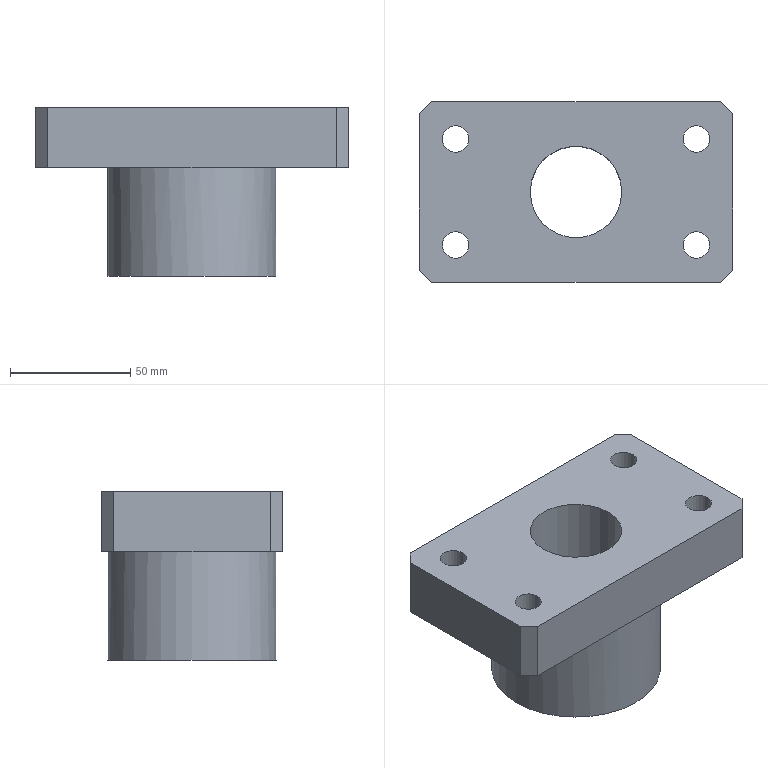Part | NX | features solid 2 | 1 solid | 17 faces | box 130 x 75 x 70 mm | volume 326789 mm3 | plane 11 | cylinder 6 | commonest cylinder face diameters 11 x4 38 x1 70 x1
STEP:
#1=CARTESIAN_POINT('',(-539.5,-198.,230.));
#2=VERTEX_POINT('',#1);
#3=CARTESIAN_POINT('',(-545.,-198.,230.));
#4=DIRECTION('',(0.,0.,1.));
#5=DIRECTION('',(1.,0.,0.));
#6=AXIS2_PLACEMENT_3D('',#3,#4,#5);
#7=CIRCLE('',#6,5.5);
#8=EDGE_CURVE('',#2,#2,#7,.T.);
#9=ORIENTED_EDGE('',*,*,#8,.F.);
#10=EDGE_LOOP('',(#9));
#11=FACE_BOUND('',#10,.T.);
#12=CARTESIAN_POINT('',(-655.,-257.5,230.));
#13=VERTEX_POINT('',#12);
#14=CARTESIAN_POINT('',(-660.,-252.5,230.));
#15=VERTEX_POINT('',#14);
#16=CARTESIAN_POINT('',(-655.,-257.5,230.));
#17=DIRECTION('',(-0.7071,0.7071,0.));
#18=VECTOR('',#17,1000.);
#19=LINE('',#16,#18);
#20=EDGE_CURVE('',#13,#15,#19,.T.);
#21=ORIENTED_EDGE('',*,*,#20,.F.);
#22=CARTESIAN_POINT('',(-535.,-257.5,230.));
#23=VERTEX_POINT('',#22);
#24=CARTESIAN_POINT('',(-535.,-257.5,230.));
#25=DIRECTION('',(-1.,0.,0.));
#26=VECTOR('',#25,1000.);
#27=LINE('',#24,#26);
#28=EDGE_CURVE('',#23,#13,#27,.T.);
#29=ORIENTED_EDGE('',*,*,#28,.F.);
#30=CARTESIAN_POINT('',(-530.,-252.5,230.));
#31=VERTEX_POINT('',#30);
#32=CARTESIAN_POINT('',(-530.,-252.5,230.));
#33=DIRECTION('',(-0.7071,-0.7071,0.));
#34=VECTOR('',#33,1000.);
#35=LINE('',#32,#34);
#36=EDGE_CURVE('',#31,#23,#35,.T.);
#37=ORIENTED_EDGE('',*,*,#36,.F.);
#38=CARTESIAN_POINT('',(-530.,-187.5,230.));
#39=VERTEX_POINT('',#38);
#40=CARTESIAN_POINT('',(-530.,-187.5,230.));
#41=DIRECTION('',(0.,-1.,0.));
#42=VECTOR('',#41,1000.);
#43=LINE('',#40,#42);
#44=EDGE_CURVE('',#39,#31,#43,.T.);
#45=ORIENTED_EDGE('',*,*,#44,.F.);
#46=CARTESIAN_POINT('',(-535.,-182.5,230.));
#47=VERTEX_POINT('',#46);
#48=CARTESIAN_POINT('',(-535.,-182.5,230.));
#49=DIRECTION('',(0.7071,-0.7071,0.));
#50=VECTOR('',#49,1000.);
#51=LINE('',#48,#50);
#52=EDGE_CURVE('',#47,#39,#51,.T.);
#53=ORIENTED_EDGE('',*,*,#52,.F.);
#54=CARTESIAN_POINT('',(-655.,-182.5,230.));
#55=VERTEX_POINT('',#54);
#56=CARTESIAN_POINT('',(-655.,-182.5,230.));
#57=DIRECTION('',(1.,0.,0.));
#58=VECTOR('',#57,1000.);
#59=LINE('',#56,#58);
#60=EDGE_CURVE('',#55,#47,#59,.T.);
#61=ORIENTED_EDGE('',*,*,#60,.F.);
#62=CARTESIAN_POINT('',(-660.,-187.5,230.));
#63=VERTEX_POINT('',#62);
#64=CARTESIAN_POINT('',(-660.,-187.5,230.));
#65=DIRECTION('',(0.7071,0.7071,0.));
#66=VECTOR('',#65,1000.);
#67=LINE('',#64,#66);
#68=EDGE_CURVE('',#63,#55,#67,.T.);
#69=ORIENTED_EDGE('',*,*,#68,.F.);
#70=CARTESIAN_POINT('',(-660.,-252.5,230.));
#71=DIRECTION('',(0.,1.,0.));
#72=VECTOR('',#71,1000.);
#73=LINE('',#70,#72);
#74=EDGE_CURVE('',#15,#63,#73,.T.);
#75=ORIENTED_EDGE('',*,*,#74,.F.);
#76=EDGE_LOOP('',(#21,#29,#37,#45,#53,#61,#69,#75));
#77=FACE_BOUND('',#76,.T.);
#78=CARTESIAN_POINT('',(-539.5,-242.,230.));
#79=VERTEX_POINT('',#78);
#80=CARTESIAN_POINT('',(-545.,-242.,230.));
#81=DIRECTION('',(0.,0.,-1.));
#82=DIRECTION('',(1.,0.,0.));
#83=AXIS2_PLACEMENT_3D('',#80,#81,#82);
#84=CIRCLE('',#83,5.5);
#85=EDGE_CURVE('',#79,#79,#84,.T.);
#86=ORIENTED_EDGE('',*,*,#85,.T.);
#87=EDGE_LOOP('',(#86));
#88=FACE_BOUND('',#87,.T.);
#89=CARTESIAN_POINT('',(-639.5,-242.,230.));
#90=VERTEX_POINT('',#89);
#91=CARTESIAN_POINT('',(-645.,-242.,230.));
#92=DIRECTION('',(0.,0.,-1.));
#93=DIRECTION('',(1.,0.,0.));
#94=AXIS2_PLACEMENT_3D('',#91,#92,#93);
#95=CIRCLE('',#94,5.5);
#96=EDGE_CURVE('',#90,#90,#95,.T.);
#97=ORIENTED_EDGE('',*,*,#96,.T.);
#98=EDGE_LOOP('',(#97));
#99=FACE_BOUND('',#98,.T.);
#100=CARTESIAN_POINT('',(-639.5,-198.,230.));
#101=VERTEX_POINT('',#100);
#102=CARTESIAN_POINT('',(-645.,-198.,230.));
#103=DIRECTION('',(0.,0.,1.));
#104=DIRECTION('',(1.,0.,0.));
#105=AXIS2_PLACEMENT_3D('',#102,#103,#104);
#106=CIRCLE('',#105,5.5);
#107=EDGE_CURVE('',#101,#101,#106,.T.);
#108=ORIENTED_EDGE('',*,*,#107,.F.);
#109=EDGE_LOOP('',(#108));
#110=FACE_BOUND('',#109,.T.);
#111=CARTESIAN_POINT('',(-576.,-220.,230.));
#112=VERTEX_POINT('',#111);
#113=CARTESIAN_POINT('',(-595.,-220.,230.));
#114=DIRECTION('',(0.,0.,1.));
#115=DIRECTION('',(1.,0.,0.));
#116=AXIS2_PLACEMENT_3D('',#113,#114,#115);
#117=CIRCLE('',#116,19.);
#118=EDGE_CURVE('',#112,#112,#117,.F.);
#119=ORIENTED_EDGE('',*,*,#118,.T.);
#120=EDGE_LOOP('',(#119));
#121=FACE_BOUND('',#120,.T.);
#122=CARTESIAN_POINT('',(-595.,-317.5,230.));
#123=DIRECTION('',(0.,0.,1.));
#124=DIRECTION('',(-1.,0.,0.));
#125=AXIS2_PLACEMENT_3D('',#122,#123,#124);
#126=PLANE('',#125);
#127=ADVANCED_FACE('',(#11,#77,#88,#99,#110,#121),#126,.T.);
#128=CARTESIAN_POINT('',(-630.,-220.,160.));
#129=VERTEX_POINT('',#128);
#130=CARTESIAN_POINT('',(-595.,-220.,160.));
#131=DIRECTION('',(0.,0.,-1.));
#132=DIRECTION('',(-1.,0.,0.));
#133=AXIS2_PLACEMENT_3D('',#130,#131,#132);
#134=CIRCLE('',#133,35.);
#135=EDGE_CURVE('',#129,#129,#134,.T.);
#136=ORIENTED_EDGE('',*,*,#135,.T.);
#137=EDGE_LOOP('',(#136));
#138=FACE_BOUND('',#137,.T.);
#139=CARTESIAN_POINT('',(-614.,-220.,160.));
#140=VERTEX_POINT('',#139);
#141=CARTESIAN_POINT('',(-595.,-220.,160.));
#142=DIRECTION('',(0.,0.,-1.));
#143=DIRECTION('',(-1.,0.,0.));
#144=AXIS2_PLACEMENT_3D('',#141,#142,#143);
#145=CIRCLE('',#144,19.);
#146=EDGE_CURVE('',#140,#140,#145,.F.);
#147=ORIENTED_EDGE('',*,*,#146,.T.);
#148=EDGE_LOOP('',(#147));
#149=FACE_BOUND('',#148,.T.);
#150=CARTESIAN_POINT('',(-595.,-220.,160.));
#151=DIRECTION('',(0.,0.,-1.));
#152=DIRECTION('',(1.,0.,0.));
#153=AXIS2_PLACEMENT_3D('',#150,#151,#152);
#154=PLANE('',#153);
#155=ADVANCED_FACE('',(#138,#149),#154,.T.);
#156=CARTESIAN_POINT('',(-639.5,-198.,205.));
#157=VERTEX_POINT('',#156);
#158=CARTESIAN_POINT('',(-645.,-198.,205.));
#159=DIRECTION('',(0.,0.,1.));
#160=DIRECTION('',(1.,0.,0.));
#161=AXIS2_PLACEMENT_3D('',#158,#159,#160);
#162=CIRCLE('',#161,5.5);
#163=EDGE_CURVE('',#157,#157,#162,.T.);
#164=ORIENTED_EDGE('',*,*,#163,.T.);
#165=EDGE_LOOP('',(#164));
#166=FACE_BOUND('',#165,.T.);
#167=CARTESIAN_POINT('',(-639.5,-242.,205.));
#168=VERTEX_POINT('',#167);
#169=CARTESIAN_POINT('',(-645.,-242.,205.));
#170=DIRECTION('',(0.,0.,-1.));
#171=DIRECTION('',(1.,0.,0.));
#172=AXIS2_PLACEMENT_3D('',#169,#170,#171);
#173=CIRCLE('',#172,5.5);
#174=EDGE_CURVE('',#168,#168,#173,.T.);
#175=ORIENTED_EDGE('',*,*,#174,.F.);
#176=EDGE_LOOP('',(#175));
#177=FACE_BOUND('',#176,.T.);
#178=CARTESIAN_POINT('',(-539.5,-242.,205.));
#179=VERTEX_POINT('',#178);
#180=CARTESIAN_POINT('',(-545.,-242.,205.));
#181=DIRECTION('',(0.,0.,-1.));
#182=DIRECTION('',(1.,0.,0.));
#183=AXIS2_PLACEMENT_3D('',#180,#181,#182);
#184=CIRCLE('',#183,5.5);
#185=EDGE_CURVE('',#179,#179,#184,.T.);
#186=ORIENTED_EDGE('',*,*,#185,.F.);
#187=EDGE_LOOP('',(#186));
#188=FACE_BOUND('',#187,.T.);
#189=CARTESIAN_POINT('',(-655.,-257.5,205.));
#190=VERTEX_POINT('',#189);
#191=CARTESIAN_POINT('',(-660.,-252.5,205.));
#192=VERTEX_POINT('',#191);
#193=CARTESIAN_POINT('',(-655.,-257.5,205.));
#194=DIRECTION('',(-0.7071,0.7071,0.));
#195=VECTOR('',#194,1000.);
#196=LINE('',#193,#195);
#197=EDGE_CURVE('',#190,#192,#196,.T.);
#198=ORIENTED_EDGE('',*,*,#197,.T.);
#199=CARTESIAN_POINT('',(-660.,-187.5,205.));
#200=VERTEX_POINT('',#199);
#201=CARTESIAN_POINT('',(-660.,-252.5,205.));
#202=DIRECTION('',(0.,1.,0.));
#203=VECTOR('',#202,1000.);
#204=LINE('',#201,#203);
#205=EDGE_CURVE('',#192,#200,#204,.T.);
#206=ORIENTED_EDGE('',*,*,#205,.T.);
#207=CARTESIAN_POINT('',(-655.,-182.5,205.));
#208=VERTEX_POINT('',#207);
#209=CARTESIAN_POINT('',(-660.,-187.5,205.));
#210=DIRECTION('',(0.7071,0.7071,0.));
#211=VECTOR('',#210,1000.);
#212=LINE('',#209,#211);
#213=EDGE_CURVE('',#200,#208,#212,.T.);
#214=ORIENTED_EDGE('',*,*,#213,.T.);
#215=CARTESIAN_POINT('',(-535.,-182.5,205.));
#216=VERTEX_POINT('',#215);
#217=CARTESIAN_POINT('',(-655.,-182.5,205.));
#218=DIRECTION('',(1.,0.,0.));
#219=VECTOR('',#218,1000.);
#220=LINE('',#217,#219);
#221=EDGE_CURVE('',#208,#216,#220,.T.);
#222=ORIENTED_EDGE('',*,*,#221,.T.);
#223=CARTESIAN_POINT('',(-530.,-187.5,205.));
#224=VERTEX_POINT('',#223);
#225=CARTESIAN_POINT('',(-535.,-182.5,205.));
#226=DIRECTION('',(0.7071,-0.7071,0.));
#227=VECTOR('',#226,1000.);
#228=LINE('',#225,#227);
#229=EDGE_CURVE('',#216,#224,#228,.T.);
#230=ORIENTED_EDGE('',*,*,#229,.T.);
#231=CARTESIAN_POINT('',(-530.,-252.5,205.));
#232=VERTEX_POINT('',#231);
#233=CARTESIAN_POINT('',(-530.,-187.5,205.));
#234=DIRECTION('',(0.,-1.,0.));
#235=VECTOR('',#234,1000.);
#236=LINE('',#233,#235);
#237=EDGE_CURVE('',#224,#232,#236,.T.);
#238=ORIENTED_EDGE('',*,*,#237,.T.);
#239=CARTESIAN_POINT('',(-535.,-257.5,205.));
#240=VERTEX_POINT('',#239);
#241=CARTESIAN_POINT('',(-530.,-252.5,205.));
#242=DIRECTION('',(-0.7071,-0.7071,0.));
#243=VECTOR('',#242,1000.);
#244=LINE('',#241,#243);
#245=EDGE_CURVE('',#232,#240,#244,.T.);
#246=ORIENTED_EDGE('',*,*,#245,.T.);
#247=CARTESIAN_POINT('',(-535.,-257.5,205.));
#248=DIRECTION('',(-1.,0.,0.));
#249=VECTOR('',#248,1000.);
#250=LINE('',#247,#249);
#251=EDGE_CURVE('',#240,#190,#250,.T.);
#252=ORIENTED_EDGE('',*,*,#251,.T.);
#253=EDGE_LOOP('',(#198,#206,#214,#222,#230,#238,#246,#252));
#254=FACE_BOUND('',#253,.T.);
#255=CARTESIAN_POINT('',(-539.5,-198.,205.));
#256=VERTEX_POINT('',#255);
#257=CARTESIAN_POINT('',(-545.,-198.,205.));
#258=DIRECTION('',(0.,0.,1.));
#259=DIRECTION('',(1.,0.,0.));
#260=AXIS2_PLACEMENT_3D('',#257,#258,#259);
#261=CIRCLE('',#260,5.5);
#262=EDGE_CURVE('',#256,#256,#261,.T.);
#263=ORIENTED_EDGE('',*,*,#262,.T.);
#264=EDGE_LOOP('',(#263));
#265=FACE_BOUND('',#264,.T.);
#266=CARTESIAN_POINT('',(-560.,-220.,205.));
#267=VERTEX_POINT('',#266);
#268=CARTESIAN_POINT('',(-595.,-220.,205.));
#269=DIRECTION('',(0.,0.,1.));
#270=DIRECTION('',(1.,0.,0.));
#271=AXIS2_PLACEMENT_3D('',#268,#269,#270);
#272=CIRCLE('',#271,35.);
#273=EDGE_CURVE('',#267,#267,#272,.F.);
#274=ORIENTED_EDGE('',*,*,#273,.F.);
#275=EDGE_LOOP('',(#274));
#276=FACE_BOUND('',#275,.T.);
#277=CARTESIAN_POINT('',(-595.,-317.5,205.));
#278=DIRECTION('',(0.,0.,1.));
#279=DIRECTION('',(-1.,0.,0.));
#280=AXIS2_PLACEMENT_3D('',#277,#278,#279);
#281=PLANE('',#280);
#282=ADVANCED_FACE('',(#166,#177,#188,#254,#265,#276),#281,.F.);
#283=ORIENTED_EDGE('',*,*,#20,.T.);
#284=CARTESIAN_POINT('',(-660.,-252.5,205.));
#285=DIRECTION('',(0.,0.,1.));
#286=VECTOR('',#285,1000.);
#287=LINE('',#284,#286);
#288=EDGE_CURVE('',#192,#15,#287,.T.);
#289=ORIENTED_EDGE('',*,*,#288,.F.);
#290=ORIENTED_EDGE('',*,*,#197,.F.);
#291=CARTESIAN_POINT('',(-655.,-257.5,205.));
#292=DIRECTION('',(0.,0.,1.));
#293=VECTOR('',#292,1000.);
#294=LINE('',#291,#293);
#295=EDGE_CURVE('',#190,#13,#294,.T.);
#296=ORIENTED_EDGE('',*,*,#295,.T.);
#297=EDGE_LOOP('',(#283,#289,#290,#296));
#298=FACE_BOUND('',#297,.T.);
#299=CARTESIAN_POINT('',(-655.,-257.5,205.));
#300=DIRECTION('',(0.7071,0.7071,0.));
#301=DIRECTION('',(0.7071,-0.7071,0.));
#302=AXIS2_PLACEMENT_3D('',#299,#300,#301);
#303=PLANE('',#302);
#304=ADVANCED_FACE('',(#298),#303,.F.);
#305=ORIENTED_EDGE('',*,*,#74,.T.);
#306=CARTESIAN_POINT('',(-660.,-187.5,205.));
#307=DIRECTION('',(0.,0.,1.));
#308=VECTOR('',#307,1000.);
#309=LINE('',#306,#308);
#310=EDGE_CURVE('',#200,#63,#309,.T.);
#311=ORIENTED_EDGE('',*,*,#310,.F.);
#312=ORIENTED_EDGE('',*,*,#205,.F.);
#313=ORIENTED_EDGE('',*,*,#288,.T.);
#314=EDGE_LOOP('',(#305,#311,#312,#313));
#315=FACE_BOUND('',#314,.T.);
#316=CARTESIAN_POINT('',(-660.,-252.5,205.));
#317=DIRECTION('',(1.,0.,0.));
#318=DIRECTION('',(0.,-1.,0.));
#319=AXIS2_PLACEMENT_3D('',#316,#317,#318);
#320=PLANE('',#319);
#321=ADVANCED_FACE('',(#315),#320,.F.);
#322=ORIENTED_EDGE('',*,*,#68,.T.);
#323=CARTESIAN_POINT('',(-655.,-182.5,205.));
#324=DIRECTION('',(0.,0.,1.));
#325=VECTOR('',#324,1000.);
#326=LINE('',#323,#325);
#327=EDGE_CURVE('',#208,#55,#326,.T.);
#328=ORIENTED_EDGE('',*,*,#327,.F.);
#329=ORIENTED_EDGE('',*,*,#213,.F.);
#330=ORIENTED_EDGE('',*,*,#310,.T.);
#331=EDGE_LOOP('',(#322,#328,#329,#330));
#332=FACE_BOUND('',#331,.T.);
#333=CARTESIAN_POINT('',(-660.,-187.5,205.));
#334=DIRECTION('',(0.7071,-0.7071,0.));
#335=DIRECTION('',(-0.7071,-0.7071,0.));
#336=AXIS2_PLACEMENT_3D('',#333,#334,#335);
#337=PLANE('',#336);
#338=ADVANCED_FACE('',(#332),#337,.F.);
#339=ORIENTED_EDGE('',*,*,#60,.T.);
#340=CARTESIAN_POINT('',(-535.,-182.5,205.));
#341=DIRECTION('',(0.,0.,1.));
#342=VECTOR('',#341,1000.);
#343=LINE('',#340,#342);
#344=EDGE_CURVE('',#216,#47,#343,.T.);
#345=ORIENTED_EDGE('',*,*,#344,.F.);
#346=ORIENTED_EDGE('',*,*,#221,.F.);
#347=ORIENTED_EDGE('',*,*,#327,.T.);
#348=EDGE_LOOP('',(#339,#345,#346,#347));
#349=FACE_BOUND('',#348,.T.);
#350=CARTESIAN_POINT('',(-655.,-182.5,205.));
#351=DIRECTION('',(0.,-1.,0.));
#352=DIRECTION('',(-1.,0.,0.));
#353=AXIS2_PLACEMENT_3D('',#350,#351,#352);
#354=PLANE('',#353);
#355=ADVANCED_FACE('',(#349),#354,.F.);
#356=ORIENTED_EDGE('',*,*,#52,.T.);
#357=CARTESIAN_POINT('',(-530.,-187.5,205.));
#358=DIRECTION('',(0.,0.,1.));
#359=VECTOR('',#358,1000.);
#360=LINE('',#357,#359);
#361=EDGE_CURVE('',#224,#39,#360,.T.);
#362=ORIENTED_EDGE('',*,*,#361,.F.);
#363=ORIENTED_EDGE('',*,*,#229,.F.);
#364=ORIENTED_EDGE('',*,*,#344,.T.);
#365=EDGE_LOOP('',(#356,#362,#363,#364));
#366=FACE_BOUND('',#365,.T.);
#367=CARTESIAN_POINT('',(-535.,-182.5,205.));
#368=DIRECTION('',(-0.7071,-0.7071,0.));
#369=DIRECTION('',(-0.7071,0.7071,0.));
#370=AXIS2_PLACEMENT_3D('',#367,#368,#369);
#371=PLANE('',#370);
#372=ADVANCED_FACE('',(#366),#371,.F.);
#373=ORIENTED_EDGE('',*,*,#44,.T.);
#374=CARTESIAN_POINT('',(-530.,-252.5,205.));
#375=DIRECTION('',(0.,0.,1.));
#376=VECTOR('',#375,1000.);
#377=LINE('',#374,#376);
#378=EDGE_CURVE('',#232,#31,#377,.T.);
#379=ORIENTED_EDGE('',*,*,#378,.F.);
#380=ORIENTED_EDGE('',*,*,#237,.F.);
#381=ORIENTED_EDGE('',*,*,#361,.T.);
#382=EDGE_LOOP('',(#373,#379,#380,#381));
#383=FACE_BOUND('',#382,.T.);
#384=CARTESIAN_POINT('',(-530.,-187.5,205.));
#385=DIRECTION('',(-1.,0.,0.));
#386=DIRECTION('',(0.,0.,-1.));
#387=AXIS2_PLACEMENT_3D('',#384,#385,#386);
#388=PLANE('',#387);
#389=ADVANCED_FACE('',(#383),#388,.F.);
#390=ORIENTED_EDGE('',*,*,#36,.T.);
#391=CARTESIAN_POINT('',(-535.,-257.5,205.));
#392=DIRECTION('',(0.,0.,1.));
#393=VECTOR('',#392,1000.);
#394=LINE('',#391,#393);
#395=EDGE_CURVE('',#240,#23,#394,.T.);
#396=ORIENTED_EDGE('',*,*,#395,.F.);
#397=ORIENTED_EDGE('',*,*,#245,.F.);
#398=ORIENTED_EDGE('',*,*,#378,.T.);
#399=EDGE_LOOP('',(#390,#396,#397,#398));
#400=FACE_BOUND('',#399,.T.);
#401=CARTESIAN_POINT('',(-530.,-252.5,205.));
#402=DIRECTION('',(-0.7071,0.7071,0.));
#403=DIRECTION('',(0.7071,0.7071,0.));
#404=AXIS2_PLACEMENT_3D('',#401,#402,#403);
#405=PLANE('',#404);
#406=ADVANCED_FACE('',(#400),#405,.F.);
#407=ORIENTED_EDGE('',*,*,#174,.T.);
#408=EDGE_LOOP('',(#407));
#409=FACE_BOUND('',#408,.T.);
#410=ORIENTED_EDGE('',*,*,#96,.F.);
#411=EDGE_LOOP('',(#410));
#412=FACE_BOUND('',#411,.T.);
#413=CARTESIAN_POINT('',(-645.,-242.,205.));
#414=DIRECTION('',(0.,0.,1.));
#415=DIRECTION('',(-1.,0.,0.));
#416=AXIS2_PLACEMENT_3D('',#413,#414,#415);
#417=CYLINDRICAL_SURFACE('',#416,5.5);
#418=ADVANCED_FACE('',(#409,#412),#417,.F.);
#419=ORIENTED_EDGE('',*,*,#185,.T.);
#420=EDGE_LOOP('',(#419));
#421=FACE_BOUND('',#420,.T.);
#422=ORIENTED_EDGE('',*,*,#85,.F.);
#423=EDGE_LOOP('',(#422));
#424=FACE_BOUND('',#423,.T.);
#425=CARTESIAN_POINT('',(-545.,-242.,205.));
#426=DIRECTION('',(0.,0.,1.));
#427=DIRECTION('',(-1.,0.,0.));
#428=AXIS2_PLACEMENT_3D('',#425,#426,#427);
#429=CYLINDRICAL_SURFACE('',#428,5.5);
#430=ADVANCED_FACE('',(#421,#424),#429,.F.);
#431=ORIENTED_EDGE('',*,*,#28,.T.);
#432=ORIENTED_EDGE('',*,*,#295,.F.);
#433=ORIENTED_EDGE('',*,*,#251,.F.);
#434=ORIENTED_EDGE('',*,*,#395,.T.);
#435=EDGE_LOOP('',(#431,#432,#433,#434));
#436=FACE_BOUND('',#435,.T.);
#437=CARTESIAN_POINT('',(-535.,-257.5,205.));
#438=DIRECTION('',(0.,1.,0.));
#439=DIRECTION('',(0.,0.,1.));
#440=AXIS2_PLACEMENT_3D('',#437,#438,#439);
#441=PLANE('',#440);
#442=ADVANCED_FACE('',(#436),#441,.F.);
#443=ORIENTED_EDGE('',*,*,#262,.F.);
#444=EDGE_LOOP('',(#443));
#445=FACE_BOUND('',#444,.T.);
#446=ORIENTED_EDGE('',*,*,#8,.T.);
#447=EDGE_LOOP('',(#446));
#448=FACE_BOUND('',#447,.T.);
#449=CARTESIAN_POINT('',(-545.,-198.,205.));
#450=DIRECTION('',(0.,0.,1.));
#451=DIRECTION('',(-1.,0.,0.));
#452=AXIS2_PLACEMENT_3D('',#449,#450,#451);
#453=CYLINDRICAL_SURFACE('',#452,5.5);
#454=ADVANCED_FACE('',(#445,#448),#453,.F.);
#455=ORIENTED_EDGE('',*,*,#163,.F.);
#456=EDGE_LOOP('',(#455));
#457=FACE_BOUND('',#456,.T.);
#458=ORIENTED_EDGE('',*,*,#107,.T.);
#459=EDGE_LOOP('',(#458));
#460=FACE_BOUND('',#459,.T.);
#461=CARTESIAN_POINT('',(-645.,-198.,205.));
#462=DIRECTION('',(0.,0.,1.));
#463=DIRECTION('',(-1.,0.,0.));
#464=AXIS2_PLACEMENT_3D('',#461,#462,#463);
#465=CYLINDRICAL_SURFACE('',#464,5.5);
#466=ADVANCED_FACE('',(#457,#460),#465,.F.);
#467=ORIENTED_EDGE('',*,*,#135,.F.);
#468=EDGE_LOOP('',(#467));
#469=FACE_BOUND('',#468,.T.);
#470=ORIENTED_EDGE('',*,*,#273,.T.);
#471=EDGE_LOOP('',(#470));
#472=FACE_BOUND('',#471,.T.);
#473=CARTESIAN_POINT('',(-595.,-220.,180.));
#474=DIRECTION('',(0.,0.,1.));
#475=DIRECTION('',(-1.,0.,0.));
#476=AXIS2_PLACEMENT_3D('',#473,#474,#475);
#477=CYLINDRICAL_SURFACE('',#476,35.);
#478=ADVANCED_FACE('',(#469,#472),#477,.T.);
#479=ORIENTED_EDGE('',*,*,#118,.F.);
#480=EDGE_LOOP('',(#479));
#481=FACE_BOUND('',#480,.T.);
#482=ORIENTED_EDGE('',*,*,#146,.F.);
#483=EDGE_LOOP('',(#482));
#484=FACE_BOUND('',#483,.T.);
#485=CARTESIAN_POINT('',(-595.,-220.,360.));
#486=DIRECTION('',(0.,0.,-1.));
#487=DIRECTION('',(-1.,0.,0.));
#488=AXIS2_PLACEMENT_3D('',#485,#486,#487);
#489=CYLINDRICAL_SURFACE('',#488,19.);
#490=ADVANCED_FACE('',(#481,#484),#489,.F.);
#491=CLOSED_SHELL('',(#127,#155,#282,#304,#321,#338,#355,#372,#389,#406,#418,#430,#442,#454,#466,#478,#490));
#492=MANIFOLD_SOLID_BREP('',#491);
#493=(LENGTH_UNIT()NAMED_UNIT(*)SI_UNIT(.MILLI.,.METRE.));
#494=UNCERTAINTY_MEASURE_WITH_UNIT(LENGTH_MEASURE(0.00001),#493,'','');
#495=(NAMED_UNIT(*)PLANE_ANGLE_UNIT()SI_UNIT($,.RADIAN.));
#496=(NAMED_UNIT(*)SI_UNIT($,.STERADIAN.)SOLID_ANGLE_UNIT());
#497=(GEOMETRIC_REPRESENTATION_CONTEXT(3)GLOBAL_UNCERTAINTY_ASSIGNED_CONTEXT((#494))GLOBAL_UNIT_ASSIGNED_CONTEXT((#493,#495,#496))REPRESENTATION_CONTEXT('',''));
#498=ADVANCED_BREP_SHAPE_REPRESENTATION('',(#492),#497);